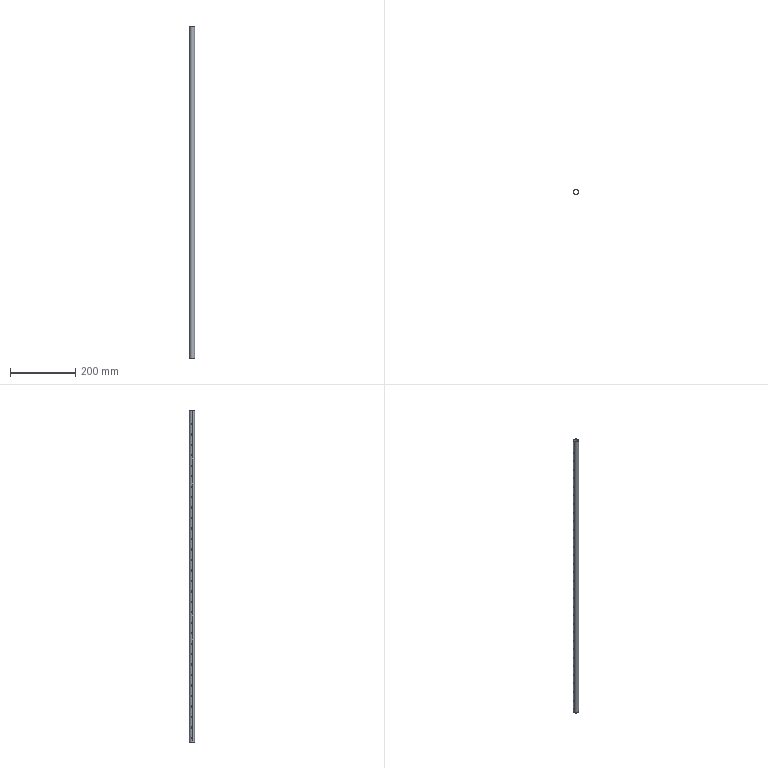Part | NX | features BREP 1 | 1 solid | 68 faces | box 16 x 16 x 1015 mm | volume 24516 mm3 | cylinder 66 | plane 2 | commonest cylinder face diameters 4 x62 15 x2 16 x2